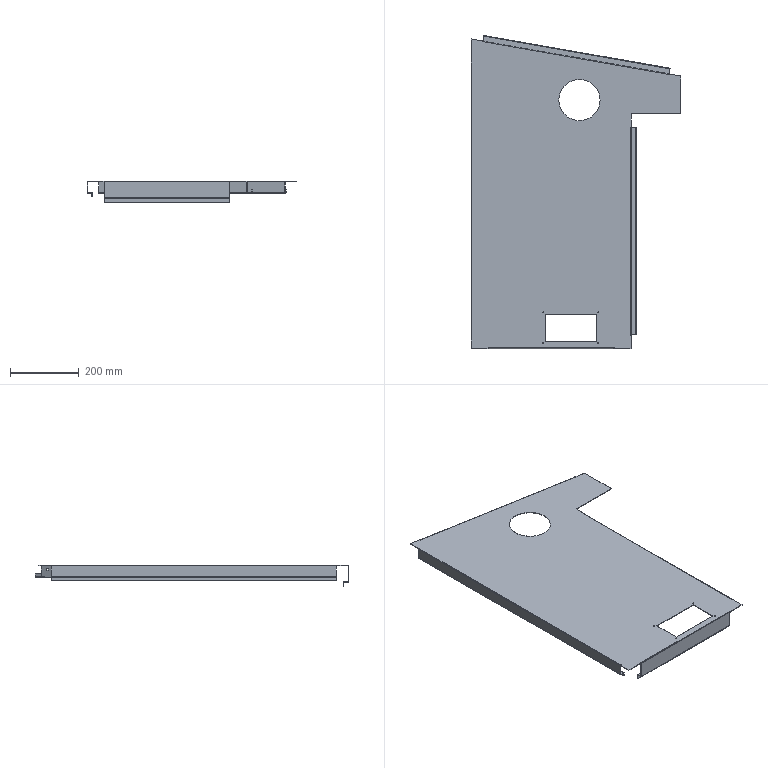Part | SolidWorks | features MirrorStock 1 | 1 solid | 160 faces | box 610 x 910.172 x 63.5 mm | volume 799310 mm3 | plane 120 | cylinder 40 | commonest cylinder face diameters 3.2 x20 0.2 x12 7 x4 4.5 x2 120 x2